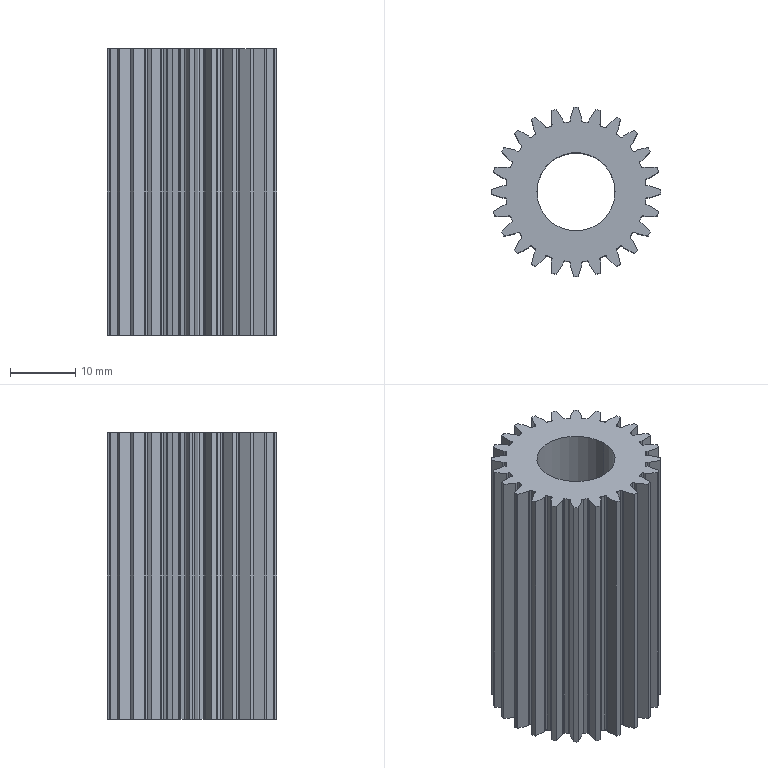Part | SolidWorks | features BaseBody 1, ICE 1 | 1 solid | 216 faces | box 26 x 26 x 44 mm | volume 14300 mm3 | cylinder 113 | plane 99 | cone 4 | commonest cylinder face diameters 0.5 x60 26 x25 21.5 x24 12 x4